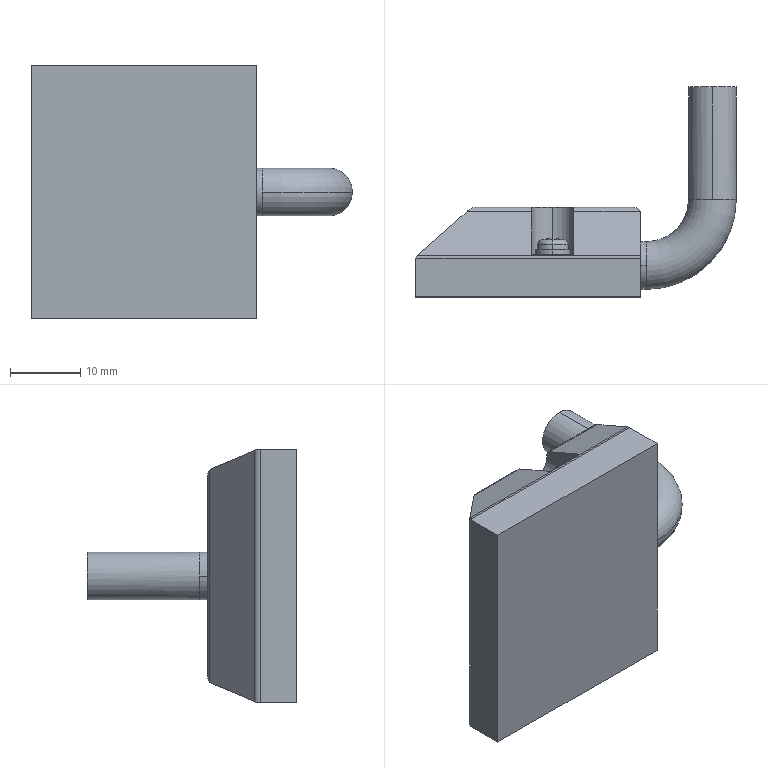Part | STEP file | Cable_Motor_Bottom_03_CM2_MSMF | 1 solid | 52 faces | box 45.598 x 29.85 x 36 mm | volume 13881 mm3 | cylinder 20 | plane 18 | torus 6 | cone 4 | sphere 4 | commonest cylinder face diameters 2 x9 5 x4 6.799 x4 6 x3